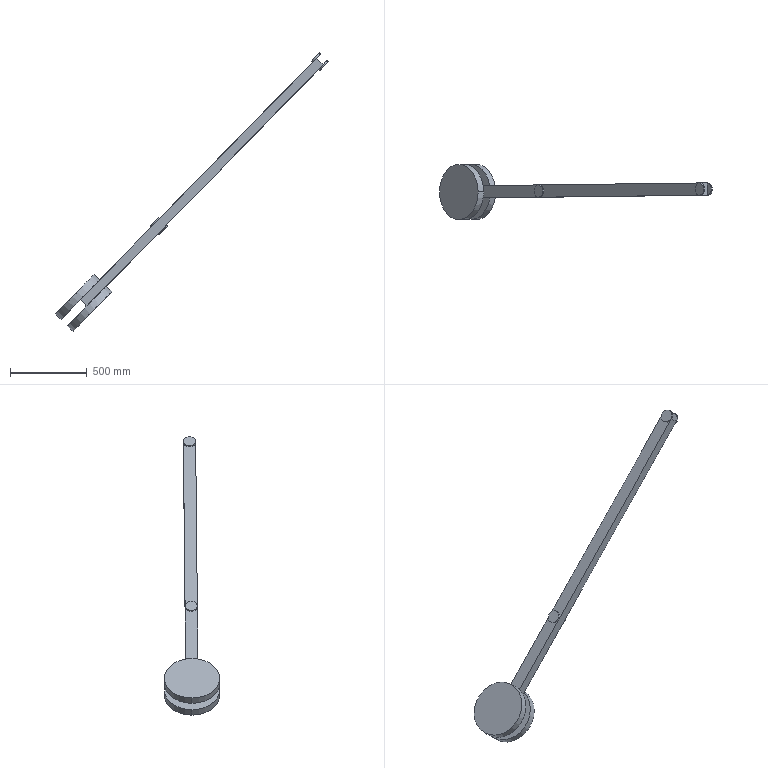Part | SolidWorks | features BaseBody 1 | 1 solid | 30 faces | box 1778 x 360 x 1813 mm | volume 20939822 mm3 | plane 18 | cylinder 12 | commonest cylinder face diameters 80 x8 360 x4
STEP:
#1=CARTESIAN_POINT('',(-992.573,1223.231,-2088.321));
#2=VERTEX_POINT('',#1);
#3=CARTESIAN_POINT('',(-1048.528,1223.231,-2145.496));
#4=VERTEX_POINT('',#3);
#5=CARTESIAN_POINT('',(-1020.55,1223.231,-2116.909));
#6=DIRECTION('',(-0.7147,0.,0.6994));
#7=DIRECTION('',(0.6994,0.,0.7147));
#8=AXIS2_PLACEMENT_3D('',#5,#6,#7);
#9=CIRCLE('',#8,40.);
#10=EDGE_CURVE('',#2,#4,#9,.T.);
#11=ORIENTED_EDGE('',*,*,#10,.T.);
#12=CARTESIAN_POINT('',(-1055.675,1223.231,-2138.502));
#13=VERTEX_POINT('',#12);
#14=CARTESIAN_POINT('',(-1048.528,1223.231,-2145.496));
#15=DIRECTION('',(-0.7147,0.,0.6994));
#16=VECTOR('',#15,1000.);
#17=LINE('',#14,#16);
#18=EDGE_CURVE('',#4,#13,#17,.T.);
#19=ORIENTED_EDGE('',*,*,#18,.T.);
#20=CARTESIAN_POINT('',(-1027.902,1263.23,-2110.124));
#21=VERTEX_POINT('',#20);
#22=CARTESIAN_POINT('',(-1027.697,1223.231,-2109.915));
#23=DIRECTION('',(0.7147,0.,-0.6994));
#24=DIRECTION('',(0.6994,0.,0.7147));
#25=AXIS2_PLACEMENT_3D('',#22,#23,#24);
#26=CIRCLE('',#25,40.);
#27=EDGE_CURVE('',#13,#21,#26,.T.);
#28=ORIENTED_EDGE('',*,*,#27,.T.);
#29=CARTESIAN_POINT('',(-999.72,1223.231,-2081.327));
#30=VERTEX_POINT('',#29);
#31=CARTESIAN_POINT('',(-1027.697,1223.231,-2109.915));
#32=DIRECTION('',(0.7147,0.,-0.6994));
#33=DIRECTION('',(0.6994,0.,0.7147));
#34=AXIS2_PLACEMENT_3D('',#31,#32,#33);
#35=CIRCLE('',#34,40.);
#36=EDGE_CURVE('',#21,#30,#35,.T.);
#37=ORIENTED_EDGE('',*,*,#36,.T.);
#38=CARTESIAN_POINT('',(-992.573,1223.231,-2088.321));
#39=DIRECTION('',(-0.7147,0.,0.6994));
#40=VECTOR('',#39,1000.);
#41=LINE('',#38,#40);
#42=EDGE_CURVE('',#2,#30,#41,.T.);
#43=ORIENTED_EDGE('',*,*,#42,.F.);
#44=EDGE_LOOP('',(#11,#19,#28,#37,#43));
#45=FACE_OUTER_BOUND('',#44,.T.);
#46=CARTESIAN_POINT('',(-1020.55,1223.231,-2116.909));
#47=DIRECTION('',(-0.7147,0.,0.6994));
#48=DIRECTION('',(0.6994,0.,0.7147));
#49=AXIS2_PLACEMENT_3D('',#46,#47,#48);
#50=CYLINDRICAL_SURFACE('',#49,40.);
#51=ADVANCED_FACE('',(#45),#50,.T.);
#52=CARTESIAN_POINT('',(56.565,1234.2,-1016.319));
#53=VERTEX_POINT('',#52);
#54=CARTESIAN_POINT('',(0.6097,1234.2,-1073.494));
#55=VERTEX_POINT('',#54);
#56=CARTESIAN_POINT('',(28.587,1234.2,-1044.906));
#57=DIRECTION('',(-0.7147,0.,0.6994));
#58=DIRECTION('',(0.6994,0.,0.7147));
#59=AXIS2_PLACEMENT_3D('',#56,#57,#58);
#60=CIRCLE('',#59,40.);
#61=EDGE_CURVE('',#53,#55,#60,.T.);
#62=ORIENTED_EDGE('',*,*,#61,.T.);
#63=CARTESIAN_POINT('',(-6.537,1234.2,-1066.5));
#64=VERTEX_POINT('',#63);
#65=CARTESIAN_POINT('',(0.6097,1234.2,-1073.494));
#66=DIRECTION('',(-0.7147,0.,0.6994));
#67=VECTOR('',#66,1000.);
#68=LINE('',#65,#67);
#69=EDGE_CURVE('',#55,#64,#68,.T.);
#70=ORIENTED_EDGE('',*,*,#69,.T.);
#71=CARTESIAN_POINT('',(21.236,1274.199,-1038.121));
#72=VERTEX_POINT('',#71);
#73=CARTESIAN_POINT('',(21.441,1234.2,-1037.912));
#74=DIRECTION('',(0.7147,0.,-0.6994));
#75=DIRECTION('',(0.6994,0.,0.7147));
#76=AXIS2_PLACEMENT_3D('',#73,#74,#75);
#77=CIRCLE('',#76,40.);
#78=EDGE_CURVE('',#64,#72,#77,.T.);
#79=ORIENTED_EDGE('',*,*,#78,.T.);
#80=CARTESIAN_POINT('',(49.418,1234.2,-1009.325));
#81=VERTEX_POINT('',#80);
#82=CARTESIAN_POINT('',(21.441,1234.2,-1037.912));
#83=DIRECTION('',(0.7147,0.,-0.6994));
#84=DIRECTION('',(0.6994,0.,0.7147));
#85=AXIS2_PLACEMENT_3D('',#82,#83,#84);
#86=CIRCLE('',#85,40.);
#87=EDGE_CURVE('',#72,#81,#86,.T.);
#88=ORIENTED_EDGE('',*,*,#87,.T.);
#89=CARTESIAN_POINT('',(56.565,1234.2,-1016.319));
#90=DIRECTION('',(-0.7147,0.,0.6994));
#91=VECTOR('',#90,1000.);
#92=LINE('',#89,#91);
#93=EDGE_CURVE('',#53,#81,#92,.T.);
#94=ORIENTED_EDGE('',*,*,#93,.F.);
#95=EDGE_LOOP('',(#62,#70,#79,#88,#94));
#96=FACE_OUTER_BOUND('',#95,.T.);
#97=CARTESIAN_POINT('',(28.587,1234.2,-1044.906));
#98=DIRECTION('',(-0.7147,0.,0.6994));
#99=DIRECTION('',(0.6994,0.,0.7147));
#100=AXIS2_PLACEMENT_3D('',#97,#98,#99);
#101=CYLINDRICAL_SURFACE('',#100,40.);
#102=ADVANCED_FACE('',(#96),#101,.T.);
#103=CARTESIAN_POINT('',(-1355.661,1218.113,-2516.511));
#104=VERTEX_POINT('',#103);
#105=CARTESIAN_POINT('',(-1607.461,1218.113,-2773.798));
#106=VERTEX_POINT('',#105);
#107=CARTESIAN_POINT('',(-1481.561,1218.113,-2645.155));
#108=DIRECTION('',(-0.7147,0.,0.6994));
#109=DIRECTION('',(0.6994,0.,0.7147));
#110=AXIS2_PLACEMENT_3D('',#107,#108,#109);
#111=CIRCLE('',#110,180.);
#112=EDGE_CURVE('',#104,#106,#111,.T.);
#113=ORIENTED_EDGE('',*,*,#112,.T.);
#114=CARTESIAN_POINT('',(-1643.195,1218.113,-2738.826));
#115=VERTEX_POINT('',#114);
#116=CARTESIAN_POINT('',(-1607.461,1218.113,-2773.798));
#117=DIRECTION('',(-0.7147,0.,0.6994));
#118=VECTOR('',#117,1000.);
#119=LINE('',#116,#118);
#120=EDGE_CURVE('',#106,#115,#119,.T.);
#121=ORIENTED_EDGE('',*,*,#120,.T.);
#122=CARTESIAN_POINT('',(-1394.751,1259.395,-2484.968));
#123=VERTEX_POINT('',#122);
#124=CARTESIAN_POINT('',(-1517.295,1218.113,-2610.182));
#125=DIRECTION('',(0.7147,0.,-0.6994));
#126=DIRECTION('',(0.6994,0.,0.7147));
#127=AXIS2_PLACEMENT_3D('',#124,#125,#126);
#128=CIRCLE('',#127,180.);
#129=EDGE_CURVE('',#115,#123,#128,.T.);
#130=ORIENTED_EDGE('',*,*,#129,.T.);
#131=CARTESIAN_POINT('',(-1391.395,1218.113,-2481.539));
#132=VERTEX_POINT('',#131);
#133=CARTESIAN_POINT('',(-1517.295,1218.113,-2610.182));
#134=DIRECTION('',(0.7147,0.,-0.6994));
#135=DIRECTION('',(0.6994,0.,0.7147));
#136=AXIS2_PLACEMENT_3D('',#133,#134,#135);
#137=CIRCLE('',#136,180.);
#138=EDGE_CURVE('',#123,#132,#137,.T.);
#139=ORIENTED_EDGE('',*,*,#138,.T.);
#140=CARTESIAN_POINT('',(-1355.661,1218.113,-2516.511));
#141=DIRECTION('',(-0.7147,0.,0.6994));
#142=VECTOR('',#141,1000.);
#143=LINE('',#140,#142);
#144=EDGE_CURVE('',#104,#132,#143,.T.);
#145=ORIENTED_EDGE('',*,*,#144,.F.);
#146=EDGE_LOOP('',(#113,#121,#130,#139,#145));
#147=FACE_OUTER_BOUND('',#146,.T.);
#148=CARTESIAN_POINT('',(-1481.561,1218.113,-2645.155));
#149=DIRECTION('',(-0.7147,0.,0.6994));
#150=DIRECTION('',(0.6994,0.,0.7147));
#151=AXIS2_PLACEMENT_3D('',#148,#149,#150);
#152=CYLINDRICAL_SURFACE('',#151,180.);
#153=ADVANCED_FACE('',(#147),#152,.T.);
#154=CARTESIAN_POINT('',(-1721.811,1218.113,-2661.887));
#155=VERTEX_POINT('',#154);
#156=CARTESIAN_POINT('',(-1470.011,1218.113,-2404.6));
#157=VERTEX_POINT('',#156);
#158=CARTESIAN_POINT('',(-1595.911,1218.113,-2533.244));
#159=DIRECTION('',(0.7147,0.,-0.6994));
#160=DIRECTION('',(-0.6994,0.,-0.7147));
#161=AXIS2_PLACEMENT_3D('',#158,#159,#160);
#162=CIRCLE('',#161,180.);
#163=EDGE_CURVE('',#155,#157,#162,.T.);
#164=ORIENTED_EDGE('',*,*,#163,.T.);
#165=CARTESIAN_POINT('',(-1434.276,1218.113,-2439.572));
#166=VERTEX_POINT('',#165);
#167=CARTESIAN_POINT('',(-1470.011,1218.113,-2404.6));
#168=DIRECTION('',(0.7147,0.,-0.6994));
#169=VECTOR('',#168,1000.);
#170=LINE('',#167,#169);
#171=EDGE_CURVE('',#157,#166,#170,.T.);
#172=ORIENTED_EDGE('',*,*,#171,.T.);
#173=CARTESIAN_POINT('',(-1437.632,1259.395,-2443.001));
#174=VERTEX_POINT('',#173);
#175=CARTESIAN_POINT('',(-1560.176,1218.113,-2568.216));
#176=DIRECTION('',(-0.7147,0.,0.6994));
#177=DIRECTION('',(-0.6994,0.,-0.7147));
#178=AXIS2_PLACEMENT_3D('',#175,#176,#177);
#179=CIRCLE('',#178,180.);
#180=EDGE_CURVE('',#166,#174,#179,.T.);
#181=ORIENTED_EDGE('',*,*,#180,.T.);
#182=CARTESIAN_POINT('',(-1686.076,1218.113,-2696.859));
#183=VERTEX_POINT('',#182);
#184=CARTESIAN_POINT('',(-1560.176,1218.113,-2568.216));
#185=DIRECTION('',(-0.7147,0.,0.6994));
#186=DIRECTION('',(-0.6994,0.,-0.7147));
#187=AXIS2_PLACEMENT_3D('',#184,#185,#186);
#188=CIRCLE('',#187,180.);
#189=EDGE_CURVE('',#174,#183,#188,.T.);
#190=ORIENTED_EDGE('',*,*,#189,.T.);
#191=CARTESIAN_POINT('',(-1721.811,1218.113,-2661.887));
#192=DIRECTION('',(0.7147,0.,-0.6994));
#193=VECTOR('',#192,1000.);
#194=LINE('',#191,#193);
#195=EDGE_CURVE('',#155,#183,#194,.T.);
#196=ORIENTED_EDGE('',*,*,#195,.F.);
#197=EDGE_LOOP('',(#164,#172,#181,#190,#196));
#198=FACE_OUTER_BOUND('',#197,.T.);
#199=CARTESIAN_POINT('',(-1595.911,1218.113,-2533.244));
#200=DIRECTION('',(0.7147,0.,-0.6994));
#201=DIRECTION('',(-0.6994,0.,-0.7147));
#202=AXIS2_PLACEMENT_3D('',#199,#200,#201);
#203=CYLINDRICAL_SURFACE('',#202,180.);
#204=ADVANCED_FACE('',(#198),#203,.T.);
#205=CARTESIAN_POINT('',(-1105.703,1223.231,-2089.541));
#206=VERTEX_POINT('',#205);
#207=CARTESIAN_POINT('',(-1049.748,1223.231,-2032.366));
#208=VERTEX_POINT('',#207);
#209=CARTESIAN_POINT('',(-1077.725,1223.231,-2060.953));
#210=DIRECTION('',(0.7147,0.,-0.6994));
#211=DIRECTION('',(-0.6994,0.,-0.7147));
#212=AXIS2_PLACEMENT_3D('',#209,#210,#211);
#213=CIRCLE('',#212,40.);
#214=EDGE_CURVE('',#206,#208,#213,.T.);
#215=ORIENTED_EDGE('',*,*,#214,.T.);
#216=CARTESIAN_POINT('',(-1042.601,1223.231,-2039.36));
#217=VERTEX_POINT('',#216);
#218=CARTESIAN_POINT('',(-1049.748,1223.231,-2032.366));
#219=DIRECTION('',(0.7147,0.,-0.6994));
#220=VECTOR('',#219,1000.);
#221=LINE('',#218,#220);
#222=EDGE_CURVE('',#208,#217,#221,.T.);
#223=ORIENTED_EDGE('',*,*,#222,.T.);
#224=CARTESIAN_POINT('',(-1070.783,1263.23,-2068.157));
#225=VERTEX_POINT('',#224);
#226=CARTESIAN_POINT('',(-1070.579,1223.231,-2067.948));
#227=DIRECTION('',(-0.7147,0.,0.6994));
#228=DIRECTION('',(-0.6994,0.,-0.7147));
#229=AXIS2_PLACEMENT_3D('',#226,#227,#228);
#230=CIRCLE('',#229,40.);
#231=EDGE_CURVE('',#217,#225,#230,.T.);
#232=ORIENTED_EDGE('',*,*,#231,.T.);
#233=CARTESIAN_POINT('',(-1098.556,1223.231,-2096.535));
#234=VERTEX_POINT('',#233);
#235=CARTESIAN_POINT('',(-1070.579,1223.231,-2067.948));
#236=DIRECTION('',(-0.7147,0.,0.6994));
#237=DIRECTION('',(-0.6994,0.,-0.7147));
#238=AXIS2_PLACEMENT_3D('',#235,#236,#237);
#239=CIRCLE('',#238,40.);
#240=EDGE_CURVE('',#225,#234,#239,.T.);
#241=ORIENTED_EDGE('',*,*,#240,.T.);
#242=CARTESIAN_POINT('',(-1105.703,1223.231,-2089.541));
#243=DIRECTION('',(0.7147,0.,-0.6994));
#244=VECTOR('',#243,1000.);
#245=LINE('',#242,#244);
#246=EDGE_CURVE('',#206,#234,#245,.T.);
#247=ORIENTED_EDGE('',*,*,#246,.F.);
#248=EDGE_LOOP('',(#215,#223,#232,#241,#247));
#249=FACE_OUTER_BOUND('',#248,.T.);
#250=CARTESIAN_POINT('',(-1077.725,1223.231,-2060.953));
#251=DIRECTION('',(0.7147,0.,-0.6994));
#252=DIRECTION('',(-0.6994,0.,-0.7147));
#253=AXIS2_PLACEMENT_3D('',#250,#251,#252);
#254=CYLINDRICAL_SURFACE('',#253,40.);
#255=ADVANCED_FACE('',(#249),#254,.T.);
#256=CARTESIAN_POINT('',(-56.565,1234.2,-1017.538));
#257=VERTEX_POINT('',#256);
#258=CARTESIAN_POINT('',(-0.6097,1234.2,-960.363));
#259=VERTEX_POINT('',#258);
#260=CARTESIAN_POINT('',(-28.587,1234.2,-988.951));
#261=DIRECTION('',(0.7147,0.,-0.6994));
#262=DIRECTION('',(-0.6994,0.,-0.7147));
#263=AXIS2_PLACEMENT_3D('',#260,#261,#262);
#264=CIRCLE('',#263,40.);
#265=EDGE_CURVE('',#257,#259,#264,.T.);
#266=ORIENTED_EDGE('',*,*,#265,.T.);
#267=CARTESIAN_POINT('',(6.537,1234.2,-967.358));
#268=VERTEX_POINT('',#267);
#269=CARTESIAN_POINT('',(-0.6097,1234.2,-960.363));
#270=DIRECTION('',(0.7147,0.,-0.6994));
#271=VECTOR('',#270,1000.);
#272=LINE('',#269,#271);
#273=EDGE_CURVE('',#259,#268,#272,.T.);
#274=ORIENTED_EDGE('',*,*,#273,.T.);
#275=CARTESIAN_POINT('',(-21.645,1274.199,-996.154));
#276=VERTEX_POINT('',#275);
#277=CARTESIAN_POINT('',(-21.441,1234.2,-995.945));
#278=DIRECTION('',(-0.7147,0.,0.6994));
#279=DIRECTION('',(-0.6994,0.,-0.7147));
#280=AXIS2_PLACEMENT_3D('',#277,#278,#279);
#281=CIRCLE('',#280,40.);
#282=EDGE_CURVE('',#268,#276,#281,.T.);
#283=ORIENTED_EDGE('',*,*,#282,.T.);
#284=CARTESIAN_POINT('',(-49.418,1234.2,-1024.533));
#285=VERTEX_POINT('',#284);
#286=CARTESIAN_POINT('',(-21.441,1234.2,-995.945));
#287=DIRECTION('',(-0.7147,0.,0.6994));
#288=DIRECTION('',(-0.6994,0.,-0.7147));
#289=AXIS2_PLACEMENT_3D('',#286,#287,#288);
#290=CIRCLE('',#289,40.);
#291=EDGE_CURVE('',#276,#285,#290,.T.);
#292=ORIENTED_EDGE('',*,*,#291,.T.);
#293=CARTESIAN_POINT('',(-56.565,1234.2,-1017.538));
#294=DIRECTION('',(0.7147,0.,-0.6994));
#295=VECTOR('',#294,1000.);
#296=LINE('',#293,#295);
#297=EDGE_CURVE('',#257,#285,#296,.T.);
#298=ORIENTED_EDGE('',*,*,#297,.F.);
#299=EDGE_LOOP('',(#266,#274,#283,#292,#298));
#300=FACE_OUTER_BOUND('',#299,.T.);
#301=CARTESIAN_POINT('',(-28.587,1234.2,-988.951));
#302=DIRECTION('',(0.7147,0.,-0.6994));
#303=DIRECTION('',(-0.6994,0.,-0.7147));
#304=AXIS2_PLACEMENT_3D('',#301,#302,#303);
#305=CYLINDRICAL_SURFACE('',#304,40.);
#306=ADVANCED_FACE('',(#300),#305,.T.);
#307=CARTESIAN_POINT('',(-1027.902,1263.23,-2110.124));
#308=DIRECTION('',(0.6994,0.007312,0.7147));
#309=VECTOR('',#308,1000.);
#310=LINE('',#307,#309);
#311=EDGE_CURVE('',#21,#72,#310,.T.);
#312=ORIENTED_EDGE('',*,*,#311,.F.);
#313=CARTESIAN_POINT('',(-1394.751,1259.395,-2484.968));
#314=DIRECTION('',(0.6994,0.007312,0.7147));
#315=VECTOR('',#314,1000.);
#316=LINE('',#313,#315);
#317=EDGE_CURVE('',#123,#21,#316,.T.);
#318=ORIENTED_EDGE('',*,*,#317,.F.);
#319=CARTESIAN_POINT('',(-1517.5,1258.112,-2610.391));
#320=VERTEX_POINT('',#319);
#321=CARTESIAN_POINT('',(-1517.5,1258.112,-2610.391));
#322=DIRECTION('',(0.6994,0.007312,0.7147));
#323=VECTOR('',#322,1000.);
#324=LINE('',#321,#323);
#325=EDGE_CURVE('',#320,#123,#324,.T.);
#326=ORIENTED_EDGE('',*,*,#325,.F.);
#327=CARTESIAN_POINT('',(-1560.381,1258.112,-2568.425));
#328=VERTEX_POINT('',#327);
#329=CARTESIAN_POINT('',(-1560.381,1258.112,-2568.425));
#330=DIRECTION('',(0.7147,0.,-0.6994));
#331=VECTOR('',#330,1000.);
#332=LINE('',#329,#331);
#333=EDGE_CURVE('',#328,#320,#332,.T.);
#334=ORIENTED_EDGE('',*,*,#333,.F.);
#335=CARTESIAN_POINT('',(-1437.632,1259.395,-2443.001));
#336=DIRECTION('',(-0.6994,-0.007312,-0.7147));
#337=VECTOR('',#336,1000.);
#338=LINE('',#335,#337);
#339=EDGE_CURVE('',#174,#328,#338,.T.);
#340=ORIENTED_EDGE('',*,*,#339,.F.);
#341=CARTESIAN_POINT('',(-1070.783,1263.23,-2068.157));
#342=DIRECTION('',(-0.6994,-0.007312,-0.7147));
#343=VECTOR('',#342,1000.);
#344=LINE('',#341,#343);
#345=EDGE_CURVE('',#225,#174,#344,.T.);
#346=ORIENTED_EDGE('',*,*,#345,.F.);
#347=CARTESIAN_POINT('',(-21.645,1274.199,-996.154));
#348=DIRECTION('',(-0.6994,-0.007312,-0.7147));
#349=VECTOR('',#348,1000.);
#350=LINE('',#347,#349);
#351=EDGE_CURVE('',#276,#225,#350,.T.);
#352=ORIENTED_EDGE('',*,*,#351,.F.);
#353=CARTESIAN_POINT('',(21.236,1274.199,-1038.121));
#354=DIRECTION('',(-0.7147,0.,0.6994));
#355=VECTOR('',#354,1000.);
#356=LINE('',#353,#355);
#357=EDGE_CURVE('',#72,#276,#356,.T.);
#358=ORIENTED_EDGE('',*,*,#357,.F.);
#359=EDGE_LOOP('',(#312,#318,#326,#334,#340,#346,#352,#358));
#360=FACE_OUTER_BOUND('',#359,.T.);
#361=CARTESIAN_POINT('',(-1517.5,1258.112,-2610.391));
#362=DIRECTION('',(0.005115,-1.,0.005226));
#363=DIRECTION('',(0.,-0.005226,-1.));
#364=AXIS2_PLACEMENT_3D('',#361,#362,#363);
#365=PLANE('',#364);
#366=ADVANCED_FACE('',(#360),#365,.F.);
#367=CARTESIAN_POINT('',(21.645,1194.201,-1037.703));
#368=VERTEX_POINT('',#367);
#369=CARTESIAN_POINT('',(21.441,1234.2,-1037.912));
#370=DIRECTION('',(0.005115,-1.,0.005226));
#371=VECTOR('',#370,1000.);
#372=LINE('',#369,#371);
#373=EDGE_CURVE('',#72,#368,#372,.T.);
#374=ORIENTED_EDGE('',*,*,#373,.F.);
#375=ORIENTED_EDGE('',*,*,#357,.T.);
#376=CARTESIAN_POINT('',(-21.236,1194.201,-995.736));
#377=VERTEX_POINT('',#376);
#378=CARTESIAN_POINT('',(-21.441,1234.2,-995.945));
#379=DIRECTION('',(-0.005115,1.,-0.005226));
#380=VECTOR('',#379,1000.);
#381=LINE('',#378,#380);
#382=EDGE_CURVE('',#377,#276,#381,.T.);
#383=ORIENTED_EDGE('',*,*,#382,.F.);
#384=CARTESIAN_POINT('',(0.2046,1194.201,-1016.72));
#385=DIRECTION('',(-0.7147,0.,0.6994));
#386=VECTOR('',#385,1000.);
#387=LINE('',#384,#386);
#388=EDGE_CURVE('',#368,#377,#387,.T.);
#389=ORIENTED_EDGE('',*,*,#388,.F.);
#390=EDGE_LOOP('',(#374,#375,#383,#389));
#391=FACE_OUTER_BOUND('',#390,.T.);
#392=CARTESIAN_POINT('',(0.,1234.2,-1016.929));
#393=DIRECTION('',(-0.6994,-0.007312,-0.7147));
#394=DIRECTION('',(-0.7147,0.,0.6994));
#395=AXIS2_PLACEMENT_3D('',#392,#393,#394);
#396=PLANE('',#395);
#397=ADVANCED_FACE('',(#391),#396,.F.);
#398=ORIENTED_EDGE('',*,*,#36,.F.);
#399=ORIENTED_EDGE('',*,*,#311,.T.);
#400=ORIENTED_EDGE('',*,*,#78,.F.);
#401=CARTESIAN_POINT('',(21.441,1234.2,-1037.912));
#402=DIRECTION('',(0.7147,0.,-0.6994));
#403=DIRECTION('',(0.6994,0.,0.7147));
#404=AXIS2_PLACEMENT_3D('',#401,#402,#403);
#405=CIRCLE('',#404,40.);
#406=EDGE_CURVE('',#368,#64,#405,.T.);
#407=ORIENTED_EDGE('',*,*,#406,.F.);
#408=CARTESIAN_POINT('',(-1027.493,1183.232,-2109.705));
#409=VERTEX_POINT('',#408);
#410=CARTESIAN_POINT('',(-1027.493,1183.232,-2109.705));
#411=DIRECTION('',(0.6994,0.007312,0.7147));
#412=VECTOR('',#411,1000.);
#413=LINE('',#410,#412);
#414=EDGE_CURVE('',#409,#368,#413,.T.);
#415=ORIENTED_EDGE('',*,*,#414,.F.);
#416=CARTESIAN_POINT('',(-1027.697,1223.231,-2109.915));
#417=DIRECTION('',(0.7147,0.,-0.6994));
#418=DIRECTION('',(0.6994,0.,0.7147));
#419=AXIS2_PLACEMENT_3D('',#416,#417,#418);
#420=CIRCLE('',#419,40.);
#421=EDGE_CURVE('',#30,#409,#420,.T.);
#422=ORIENTED_EDGE('',*,*,#421,.F.);
#423=EDGE_LOOP('',(#398,#399,#400,#407,#415,#422));
#424=FACE_OUTER_BOUND('',#423,.T.);
#425=CARTESIAN_POINT('',(-1517.09,1178.114,-2609.973));
#426=DIRECTION('',(-0.7147,0.,0.6994));
#427=DIRECTION('',(0.6994,0.,0.7147));
#428=AXIS2_PLACEMENT_3D('',#425,#426,#427);
#429=PLANE('',#428);
#430=ADVANCED_FACE('',(#424),#429,.F.);
#431=CARTESIAN_POINT('',(-1027.697,1223.231,-2109.915));
#432=DIRECTION('',(0.7147,0.,-0.6994));
#433=DIRECTION('',(0.6994,0.,0.7147));
#434=AXIS2_PLACEMENT_3D('',#431,#432,#433);
#435=CIRCLE('',#434,40.);
#436=EDGE_CURVE('',#409,#13,#435,.T.);
#437=ORIENTED_EDGE('',*,*,#436,.F.);
#438=CARTESIAN_POINT('',(-1394.342,1179.397,-2484.55));
#439=VERTEX_POINT('',#438);
#440=CARTESIAN_POINT('',(-1394.342,1179.397,-2484.55));
#441=DIRECTION('',(0.6994,0.007312,0.7147));
#442=VECTOR('',#441,1000.);
#443=LINE('',#440,#442);
#444=EDGE_CURVE('',#439,#409,#443,.T.);
#445=ORIENTED_EDGE('',*,*,#444,.F.);
#446=CARTESIAN_POINT('',(-1517.295,1218.113,-2610.182));
#447=DIRECTION('',(0.7147,0.,-0.6994));
#448=DIRECTION('',(0.6994,0.,0.7147));
#449=AXIS2_PLACEMENT_3D('',#446,#447,#448);
#450=CIRCLE('',#449,180.);
#451=EDGE_CURVE('',#132,#439,#450,.T.);
#452=ORIENTED_EDGE('',*,*,#451,.F.);
#453=ORIENTED_EDGE('',*,*,#138,.F.);
#454=ORIENTED_EDGE('',*,*,#317,.T.);
#455=ORIENTED_EDGE('',*,*,#27,.F.);
#456=EDGE_LOOP('',(#437,#445,#452,#453,#454,#455));
#457=FACE_OUTER_BOUND('',#456,.T.);
#458=CARTESIAN_POINT('',(-1517.09,1178.114,-2609.973));
#459=DIRECTION('',(-0.7147,0.,0.6994));
#460=DIRECTION('',(0.6994,0.,0.7147));
#461=AXIS2_PLACEMENT_3D('',#458,#459,#460);
#462=PLANE('',#461);
#463=ADVANCED_FACE('',(#457),#462,.F.);
#464=CARTESIAN_POINT('',(-1517.09,1178.114,-2609.973));
#465=VERTEX_POINT('',#464);
#466=CARTESIAN_POINT('',(-1517.5,1258.112,-2610.391));
#467=DIRECTION('',(0.005115,-1.,0.005226));
#468=VECTOR('',#467,1000.);
#469=LINE('',#466,#468);
#470=EDGE_CURVE('',#320,#465,#469,.T.);
#471=ORIENTED_EDGE('',*,*,#470,.F.);
#472=ORIENTED_EDGE('',*,*,#325,.T.);
#473=ORIENTED_EDGE('',*,*,#129,.F.);
#474=CARTESIAN_POINT('',(-1517.295,1218.113,-2610.182));
#475=DIRECTION('',(0.7147,0.,-0.6994));
#476=DIRECTION('',(0.6994,0.,0.7147));
#477=AXIS2_PLACEMENT_3D('',#474,#475,#476);
#478=CIRCLE('',#477,180.);
#479=EDGE_CURVE('',#439,#115,#478,.T.);
#480=ORIENTED_EDGE('',*,*,#479,.F.);
#481=CARTESIAN_POINT('',(-1517.09,1178.114,-2609.973));
#482=DIRECTION('',(0.6994,0.007312,0.7147));
#483=VECTOR('',#482,1000.);
#484=LINE('',#481,#483);
#485=EDGE_CURVE('',#465,#439,#484,.T.);
#486=ORIENTED_EDGE('',*,*,#485,.F.);
#487=EDGE_LOOP('',(#471,#472,#473,#480,#486));
#488=FACE_OUTER_BOUND('',#487,.T.);
#489=CARTESIAN_POINT('',(-1517.295,1218.113,-2610.182));
#490=DIRECTION('',(0.7147,0.,-0.6994));
#491=DIRECTION('',(-0.6994,0.,-0.7147));
#492=AXIS2_PLACEMENT_3D('',#489,#490,#491);
#493=PLANE('',#492);
#494=ADVANCED_FACE('',(#488),#493,.F.);
#495=ORIENTED_EDGE('',*,*,#333,.T.);
#496=ORIENTED_EDGE('',*,*,#470,.T.);
#497=CARTESIAN_POINT('',(-1559.972,1178.114,-2568.007));
#498=VERTEX_POINT('',#497);
#499=CARTESIAN_POINT('',(-1538.531,1178.114,-2588.99));
#500=DIRECTION('',(-0.7147,0.,0.6994));
#501=VECTOR('',#500,1000.);
#502=LINE('',#499,#501);
#503=EDGE_CURVE('',#465,#498,#502,.T.);
#504=ORIENTED_EDGE('',*,*,#503,.T.);
#505=CARTESIAN_POINT('',(-1560.176,1218.113,-2568.216));
#506=DIRECTION('',(-0.005115,1.,-0.005226));
#507=VECTOR('',#506,1000.);
#508=LINE('',#505,#507);
#509=EDGE_CURVE('',#498,#328,#508,.T.);
#510=ORIENTED_EDGE('',*,*,#509,.T.);
#511=EDGE_LOOP('',(#495,#496,#504,#510));
#512=FACE_OUTER_BOUND('',#511,.T.);
#513=CARTESIAN_POINT('',(-1538.736,1218.113,-2589.199));
#514=DIRECTION('',(-0.6994,-0.007312,-0.7147));
#515=DIRECTION('',(-0.7147,0.,0.6994));
#516=AXIS2_PLACEMENT_3D('',#513,#514,#515);
#517=PLANE('',#516);
#518=ADVANCED_FACE('',(#512),#517,.T.);
#519=ORIENTED_EDGE('',*,*,#509,.F.);
#520=CARTESIAN_POINT('',(-1437.223,1179.397,-2442.583));
#521=VERTEX_POINT('',#520);
#522=CARTESIAN_POINT('',(-1437.223,1179.397,-2442.583));
#523=DIRECTION('',(-0.6994,-0.007312,-0.7147));
#524=VECTOR('',#523,1000.);
#525=LINE('',#522,#524);
#526=EDGE_CURVE('',#521,#498,#525,.T.);
#527=ORIENTED_EDGE('',*,*,#526,.F.);
#528=CARTESIAN_POINT('',(-1560.176,1218.113,-2568.216));
#529=DIRECTION('',(-0.7147,0.,0.6994));
#530=DIRECTION('',(-0.6994,0.,-0.7147));
#531=AXIS2_PLACEMENT_3D('',#528,#529,#530);
#532=CIRCLE('',#531,180.);
#533=EDGE_CURVE('',#183,#521,#532,.T.);
#534=ORIENTED_EDGE('',*,*,#533,.F.);
#535=ORIENTED_EDGE('',*,*,#189,.F.);
#536=ORIENTED_EDGE('',*,*,#339,.T.);
#537=EDGE_LOOP('',(#519,#527,#534,#535,#536));
#538=FACE_OUTER_BOUND('',#537,.T.);
#539=CARTESIAN_POINT('',(-1560.176,1218.113,-2568.216));
#540=DIRECTION('',(-0.7147,0.,0.6994));
#541=DIRECTION('',(0.6994,0.,0.7147));
#542=AXIS2_PLACEMENT_3D('',#539,#540,#541);
#543=PLANE('',#542);
#544=ADVANCED_FACE('',(#538),#543,.F.);
#545=ORIENTED_EDGE('',*,*,#345,.T.);
#546=ORIENTED_EDGE('',*,*,#180,.F.);
#547=CARTESIAN_POINT('',(-1560.176,1218.113,-2568.216));
#548=DIRECTION('',(-0.7147,0.,0.6994));
#549=DIRECTION('',(-0.6994,0.,-0.7147));
#550=AXIS2_PLACEMENT_3D('',#547,#548,#549);
#551=CIRCLE('',#550,180.);
#552=EDGE_CURVE('',#521,#166,#551,.T.);
#553=ORIENTED_EDGE('',*,*,#552,.F.);
#554=CARTESIAN_POINT('',(-1070.374,1183.232,-2067.739));
#555=VERTEX_POINT('',#554);
#556=CARTESIAN_POINT('',(-1070.374,1183.232,-2067.739));
#557=DIRECTION('',(-0.6994,-0.007312,-0.7147));
#558=VECTOR('',#557,1000.);
#559=LINE('',#556,#558);
#560=EDGE_CURVE('',#555,#521,#559,.T.);
#561=ORIENTED_EDGE('',*,*,#560,.F.);
#562=CARTESIAN_POINT('',(-1070.579,1223.231,-2067.948));
#563=DIRECTION('',(-0.7147,0.,0.6994));
#564=DIRECTION('',(-0.6994,0.,-0.7147));
#565=AXIS2_PLACEMENT_3D('',#562,#563,#564);
#566=CIRCLE('',#565,40.);
#567=EDGE_CURVE('',#234,#555,#566,.T.);
#568=ORIENTED_EDGE('',*,*,#567,.F.);
#569=ORIENTED_EDGE('',*,*,#240,.F.);
#570=EDGE_LOOP('',(#545,#546,#553,#561,#568,#569));
#571=FACE_OUTER_BOUND('',#570,.T.);
#572=CARTESIAN_POINT('',(-1559.972,1178.114,-2568.007));
#573=DIRECTION('',(0.7147,0.,-0.6994));
#574=DIRECTION('',(-0.6994,0.,-0.7147));
#575=AXIS2_PLACEMENT_3D('',#572,#573,#574);
#576=PLANE('',#575);
#577=ADVANCED_FACE('',(#571),#576,.F.);
#578=CARTESIAN_POINT('',(-21.236,1194.201,-995.736));
#579=DIRECTION('',(-0.6994,-0.007312,-0.7147));
#580=VECTOR('',#579,1000.);
#581=LINE('',#578,#580);
#582=EDGE_CURVE('',#377,#555,#581,.T.);
#583=ORIENTED_EDGE('',*,*,#582,.F.);
#584=CARTESIAN_POINT('',(-21.441,1234.2,-995.945));
#585=DIRECTION('',(-0.7147,0.,0.6994));
#586=DIRECTION('',(-0.6994,0.,-0.7147));
#587=AXIS2_PLACEMENT_3D('',#584,#585,#586);
#588=CIRCLE('',#587,40.);
#589=EDGE_CURVE('',#285,#377,#588,.T.);
#590=ORIENTED_EDGE('',*,*,#589,.F.);
#591=ORIENTED_EDGE('',*,*,#291,.F.);
#592=ORIENTED_EDGE('',*,*,#351,.T.);
#593=ORIENTED_EDGE('',*,*,#231,.F.);
#594=CARTESIAN_POINT('',(-1070.579,1223.231,-2067.948));
#595=DIRECTION('',(-0.7147,0.,0.6994));
#596=DIRECTION('',(-0.6994,0.,-0.7147));
#597=AXIS2_PLACEMENT_3D('',#594,#595,#596);
#598=CIRCLE('',#597,40.);
#599=EDGE_CURVE('',#555,#217,#598,.T.);
#600=ORIENTED_EDGE('',*,*,#599,.F.);
#601=EDGE_LOOP('',(#583,#590,#591,#592,#593,#600));
#602=FACE_OUTER_BOUND('',#601,.T.);
#603=CARTESIAN_POINT('',(-1559.972,1178.114,-2568.007));
#604=DIRECTION('',(0.7147,0.,-0.6994));
#605=DIRECTION('',(-0.6994,0.,-0.7147));
#606=AXIS2_PLACEMENT_3D('',#603,#604,#605);
#607=PLANE('',#606);
#608=ADVANCED_FACE('',(#602),#607,.F.);
#609=ORIENTED_EDGE('',*,*,#582,.T.);
#610=ORIENTED_EDGE('',*,*,#560,.T.);
#611=ORIENTED_EDGE('',*,*,#526,.T.);
#612=ORIENTED_EDGE('',*,*,#503,.F.);
#613=ORIENTED_EDGE('',*,*,#485,.T.);
#614=ORIENTED_EDGE('',*,*,#444,.T.);
#615=ORIENTED_EDGE('',*,*,#414,.T.);
#616=ORIENTED_EDGE('',*,*,#388,.T.);
#617=EDGE_LOOP('',(#609,#610,#611,#612,#613,#614,#615,#616));
#618=FACE_OUTER_BOUND('',#617,.T.);
#619=CARTESIAN_POINT('',(-1517.09,1178.114,-2609.973));
#620=DIRECTION('',(-0.005115,1.,-0.005226));
#621=DIRECTION('',(0.,0.005226,1.));
#622=AXIS2_PLACEMENT_3D('',#619,#620,#621);
#623=PLANE('',#622);
#624=ADVANCED_FACE('',(#618),#623,.F.);
#625=ORIENTED_EDGE('',*,*,#87,.F.);
#626=ORIENTED_EDGE('',*,*,#373,.T.);
#627=CARTESIAN_POINT('',(21.441,1234.2,-1037.912));
#628=DIRECTION('',(0.7147,0.,-0.6994));
#629=DIRECTION('',(0.6994,0.,0.7147));
#630=AXIS2_PLACEMENT_3D('',#627,#628,#629);
#631=CIRCLE('',#630,40.);
#632=EDGE_CURVE('',#81,#368,#631,.T.);
#633=ORIENTED_EDGE('',*,*,#632,.F.);
#634=EDGE_LOOP('',(#625,#626,#633));
#635=FACE_OUTER_BOUND('',#634,.T.);
#636=CARTESIAN_POINT('',(21.441,1234.2,-1037.912));
#637=DIRECTION('',(0.7147,0.,-0.6994));
#638=DIRECTION('',(-0.6994,0.,-0.7147));
#639=AXIS2_PLACEMENT_3D('',#636,#637,#638);
#640=PLANE('',#639);
#641=ADVANCED_FACE('',(#635),#640,.F.);
#642=ORIENTED_EDGE('',*,*,#382,.T.);
#643=ORIENTED_EDGE('',*,*,#282,.F.);
#644=CARTESIAN_POINT('',(-21.441,1234.2,-995.945));
#645=DIRECTION('',(-0.7147,0.,0.6994));
#646=DIRECTION('',(-0.6994,0.,-0.7147));
#647=AXIS2_PLACEMENT_3D('',#644,#645,#646);
#648=CIRCLE('',#647,40.);
#649=EDGE_CURVE('',#377,#268,#648,.T.);
#650=ORIENTED_EDGE('',*,*,#649,.F.);
#651=EDGE_LOOP('',(#642,#643,#650));
#652=FACE_OUTER_BOUND('',#651,.T.);
#653=CARTESIAN_POINT('',(-21.441,1234.2,-995.945));
#654=DIRECTION('',(-0.7147,0.,0.6994));
#655=DIRECTION('',(0.6994,0.,0.7147));
#656=AXIS2_PLACEMENT_3D('',#653,#654,#655);
#657=PLANE('',#656);
#658=ADVANCED_FACE('',(#652),#657,.F.);
#659=ORIENTED_EDGE('',*,*,#18,.F.);
#660=CARTESIAN_POINT('',(-1020.55,1223.231,-2116.909));
#661=DIRECTION('',(-0.7147,0.,0.6994));
#662=DIRECTION('',(0.6994,0.,0.7147));
#663=AXIS2_PLACEMENT_3D('',#660,#661,#662);
#664=CIRCLE('',#663,40.);
#665=EDGE_CURVE('',#4,#2,#664,.T.);
#666=ORIENTED_EDGE('',*,*,#665,.T.);
#667=ORIENTED_EDGE('',*,*,#42,.T.);
#668=ORIENTED_EDGE('',*,*,#421,.T.);
#669=ORIENTED_EDGE('',*,*,#436,.T.);
#670=EDGE_LOOP('',(#659,#666,#667,#668,#669));
#671=FACE_OUTER_BOUND('',#670,.T.);
#672=CARTESIAN_POINT('',(-1020.55,1223.231,-2116.909));
#673=DIRECTION('',(-0.7147,0.,0.6994));
#674=DIRECTION('',(0.6994,0.,0.7147));
#675=AXIS2_PLACEMENT_3D('',#672,#673,#674);
#676=CYLINDRICAL_SURFACE('',#675,40.);
#677=ADVANCED_FACE('',(#671),#676,.T.);
#678=ORIENTED_EDGE('',*,*,#69,.F.);
#679=CARTESIAN_POINT('',(28.587,1234.2,-1044.906));
#680=DIRECTION('',(-0.7147,0.,0.6994));
#681=DIRECTION('',(0.6994,0.,0.7147));
#682=AXIS2_PLACEMENT_3D('',#679,#680,#681);
#683=CIRCLE('',#682,40.);
#684=EDGE_CURVE('',#55,#53,#683,.T.);
#685=ORIENTED_EDGE('',*,*,#684,.T.);
#686=ORIENTED_EDGE('',*,*,#93,.T.);
#687=ORIENTED_EDGE('',*,*,#632,.T.);
#688=ORIENTED_EDGE('',*,*,#406,.T.);
#689=EDGE_LOOP('',(#678,#685,#686,#687,#688));
#690=FACE_OUTER_BOUND('',#689,.T.);
#691=CARTESIAN_POINT('',(28.587,1234.2,-1044.906));
#692=DIRECTION('',(-0.7147,0.,0.6994));
#693=DIRECTION('',(0.6994,0.,0.7147));
#694=AXIS2_PLACEMENT_3D('',#691,#692,#693);
#695=CYLINDRICAL_SURFACE('',#694,40.);
#696=ADVANCED_FACE('',(#690),#695,.T.);
#697=ORIENTED_EDGE('',*,*,#120,.F.);
#698=CARTESIAN_POINT('',(-1481.561,1218.113,-2645.155));
#699=DIRECTION('',(-0.7147,0.,0.6994));
#700=DIRECTION('',(0.6994,0.,0.7147));
#701=AXIS2_PLACEMENT_3D('',#698,#699,#700);
#702=CIRCLE('',#701,180.);
#703=EDGE_CURVE('',#106,#104,#702,.T.);
#704=ORIENTED_EDGE('',*,*,#703,.T.);
#705=ORIENTED_EDGE('',*,*,#144,.T.);
#706=ORIENTED_EDGE('',*,*,#451,.T.);
#707=ORIENTED_EDGE('',*,*,#479,.T.);
#708=EDGE_LOOP('',(#697,#704,#705,#706,#707));
#709=FACE_OUTER_BOUND('',#708,.T.);
#710=CARTESIAN_POINT('',(-1481.561,1218.113,-2645.155));
#711=DIRECTION('',(-0.7147,0.,0.6994));
#712=DIRECTION('',(0.6994,0.,0.7147));
#713=AXIS2_PLACEMENT_3D('',#710,#711,#712);
#714=CYLINDRICAL_SURFACE('',#713,180.);
#715=ADVANCED_FACE('',(#709),#714,.T.);
#716=ORIENTED_EDGE('',*,*,#171,.F.);
#717=CARTESIAN_POINT('',(-1595.911,1218.113,-2533.244));
#718=DIRECTION('',(0.7147,0.,-0.6994));
#719=DIRECTION('',(-0.6994,0.,-0.7147));
#720=AXIS2_PLACEMENT_3D('',#717,#718,#719);
#721=CIRCLE('',#720,180.);
#722=EDGE_CURVE('',#157,#155,#721,.T.);
#723=ORIENTED_EDGE('',*,*,#722,.T.);
#724=ORIENTED_EDGE('',*,*,#195,.T.);
#725=ORIENTED_EDGE('',*,*,#533,.T.);
#726=ORIENTED_EDGE('',*,*,#552,.T.);
#727=EDGE_LOOP('',(#716,#723,#724,#725,#726));
#728=FACE_OUTER_BOUND('',#727,.T.);
#729=CARTESIAN_POINT('',(-1595.911,1218.113,-2533.244));
#730=DIRECTION('',(0.7147,0.,-0.6994));
#731=DIRECTION('',(-0.6994,0.,-0.7147));
#732=AXIS2_PLACEMENT_3D('',#729,#730,#731);
#733=CYLINDRICAL_SURFACE('',#732,180.);
#734=ADVANCED_FACE('',(#728),#733,.T.);
#735=ORIENTED_EDGE('',*,*,#222,.F.);
#736=CARTESIAN_POINT('',(-1077.725,1223.231,-2060.953));
#737=DIRECTION('',(0.7147,0.,-0.6994));
#738=DIRECTION('',(-0.6994,0.,-0.7147));
#739=AXIS2_PLACEMENT_3D('',#736,#737,#738);
#740=CIRCLE('',#739,40.);
#741=EDGE_CURVE('',#208,#206,#740,.T.);
#742=ORIENTED_EDGE('',*,*,#741,.T.);
#743=ORIENTED_EDGE('',*,*,#246,.T.);
#744=ORIENTED_EDGE('',*,*,#567,.T.);
#745=ORIENTED_EDGE('',*,*,#599,.T.);
#746=EDGE_LOOP('',(#735,#742,#743,#744,#745));
#747=FACE_OUTER_BOUND('',#746,.T.);
#748=CARTESIAN_POINT('',(-1077.725,1223.231,-2060.953));
#749=DIRECTION('',(0.7147,0.,-0.6994));
#750=DIRECTION('',(-0.6994,0.,-0.7147));
#751=AXIS2_PLACEMENT_3D('',#748,#749,#750);
#752=CYLINDRICAL_SURFACE('',#751,40.);
#753=ADVANCED_FACE('',(#747),#752,.T.);
#754=ORIENTED_EDGE('',*,*,#273,.F.);
#755=CARTESIAN_POINT('',(-28.587,1234.2,-988.951));
#756=DIRECTION('',(0.7147,0.,-0.6994));
#757=DIRECTION('',(-0.6994,0.,-0.7147));
#758=AXIS2_PLACEMENT_3D('',#755,#756,#757);
#759=CIRCLE('',#758,40.);
#760=EDGE_CURVE('',#259,#257,#759,.T.);
#761=ORIENTED_EDGE('',*,*,#760,.T.);
#762=ORIENTED_EDGE('',*,*,#297,.T.);
#763=ORIENTED_EDGE('',*,*,#589,.T.);
#764=ORIENTED_EDGE('',*,*,#649,.T.);
#765=EDGE_LOOP('',(#754,#761,#762,#763,#764));
#766=FACE_OUTER_BOUND('',#765,.T.);
#767=CARTESIAN_POINT('',(-28.587,1234.2,-988.951));
#768=DIRECTION('',(0.7147,0.,-0.6994));
#769=DIRECTION('',(-0.6994,0.,-0.7147));
#770=AXIS2_PLACEMENT_3D('',#767,#768,#769);
#771=CYLINDRICAL_SURFACE('',#770,40.);
#772=ADVANCED_FACE('',(#766),#771,.T.);
#773=ORIENTED_EDGE('',*,*,#10,.F.);
#774=ORIENTED_EDGE('',*,*,#665,.F.);
#775=EDGE_LOOP('',(#773,#774));
#776=FACE_OUTER_BOUND('',#775,.T.);
#777=CARTESIAN_POINT('',(-1020.55,1223.231,-2116.909));
#778=DIRECTION('',(0.7147,0.,-0.6994));
#779=DIRECTION('',(-0.6994,0.,-0.7147));
#780=AXIS2_PLACEMENT_3D('',#777,#778,#779);
#781=PLANE('',#780);
#782=ADVANCED_FACE('',(#776),#781,.T.);
#783=ORIENTED_EDGE('',*,*,#61,.F.);
#784=ORIENTED_EDGE('',*,*,#684,.F.);
#785=EDGE_LOOP('',(#783,#784));
#786=FACE_OUTER_BOUND('',#785,.T.);
#787=CARTESIAN_POINT('',(28.587,1234.2,-1044.906));
#788=DIRECTION('',(0.7147,0.,-0.6994));
#789=DIRECTION('',(-0.6994,0.,-0.7147));
#790=AXIS2_PLACEMENT_3D('',#787,#788,#789);
#791=PLANE('',#790);
#792=ADVANCED_FACE('',(#786),#791,.T.);
#793=ORIENTED_EDGE('',*,*,#112,.F.);
#794=ORIENTED_EDGE('',*,*,#703,.F.);
#795=EDGE_LOOP('',(#793,#794));
#796=FACE_OUTER_BOUND('',#795,.T.);
#797=CARTESIAN_POINT('',(-1481.561,1218.113,-2645.155));
#798=DIRECTION('',(0.7147,0.,-0.6994));
#799=DIRECTION('',(-0.6994,0.,-0.7147));
#800=AXIS2_PLACEMENT_3D('',#797,#798,#799);
#801=PLANE('',#800);
#802=ADVANCED_FACE('',(#796),#801,.T.);
#803=ORIENTED_EDGE('',*,*,#163,.F.);
#804=ORIENTED_EDGE('',*,*,#722,.F.);
#805=EDGE_LOOP('',(#803,#804));
#806=FACE_OUTER_BOUND('',#805,.T.);
#807=CARTESIAN_POINT('',(-1595.911,1218.113,-2533.244));
#808=DIRECTION('',(-0.7147,0.,0.6994));
#809=DIRECTION('',(0.6994,0.,0.7147));
#810=AXIS2_PLACEMENT_3D('',#807,#808,#809);
#811=PLANE('',#810);
#812=ADVANCED_FACE('',(#806),#811,.T.);
#813=ORIENTED_EDGE('',*,*,#214,.F.);
#814=ORIENTED_EDGE('',*,*,#741,.F.);
#815=EDGE_LOOP('',(#813,#814));
#816=FACE_OUTER_BOUND('',#815,.T.);
#817=CARTESIAN_POINT('',(-1077.725,1223.231,-2060.953));
#818=DIRECTION('',(-0.7147,0.,0.6994));
#819=DIRECTION('',(0.6994,0.,0.7147));
#820=AXIS2_PLACEMENT_3D('',#817,#818,#819);
#821=PLANE('',#820);
#822=ADVANCED_FACE('',(#816),#821,.T.);
#823=ORIENTED_EDGE('',*,*,#265,.F.);
#824=ORIENTED_EDGE('',*,*,#760,.F.);
#825=EDGE_LOOP('',(#823,#824));
#826=FACE_OUTER_BOUND('',#825,.T.);
#827=CARTESIAN_POINT('',(-28.587,1234.2,-988.951));
#828=DIRECTION('',(-0.7147,0.,0.6994));
#829=DIRECTION('',(0.6994,0.,0.7147));
#830=AXIS2_PLACEMENT_3D('',#827,#828,#829);
#831=PLANE('',#830);
#832=ADVANCED_FACE('',(#826),#831,.T.);
#833=CLOSED_SHELL('',(#51,#102,#153,#204,#255,#306,#366,#397,#430,#463,#494,#518,#544,#577,#608,#624,#641,#658,#677,#696,#715,#734,#753,#772,#782,#792,#802,#812,#822,#832));
#834=MANIFOLD_SOLID_BREP('',#833);
#835=CARTESIAN_POINT('',(0.,0.,0.));
#836=DIRECTION('',(0.,0.,1.));
#837=DIRECTION('',(1.,0.,0.));
#838=AXIS2_PLACEMENT_3D('',#835,#836,#837);
#839=(LENGTH_UNIT()NAMED_UNIT(*)SI_UNIT(.MILLI.,.METRE.));
#840=UNCERTAINTY_MEASURE_WITH_UNIT(LENGTH_MEASURE(0.00001),#839,'','');
#841=(NAMED_UNIT(*)PLANE_ANGLE_UNIT()SI_UNIT($,.RADIAN.));
#842=(NAMED_UNIT(*)SI_UNIT($,.STERADIAN.)SOLID_ANGLE_UNIT());
#843=(GEOMETRIC_REPRESENTATION_CONTEXT(3)GLOBAL_UNCERTAINTY_ASSIGNED_CONTEXT((#840))GLOBAL_UNIT_ASSIGNED_CONTEXT((#839,#841,#842))REPRESENTATION_CONTEXT('',''));
#844=ADVANCED_BREP_SHAPE_REPRESENTATION('',(#834,#838),#843);